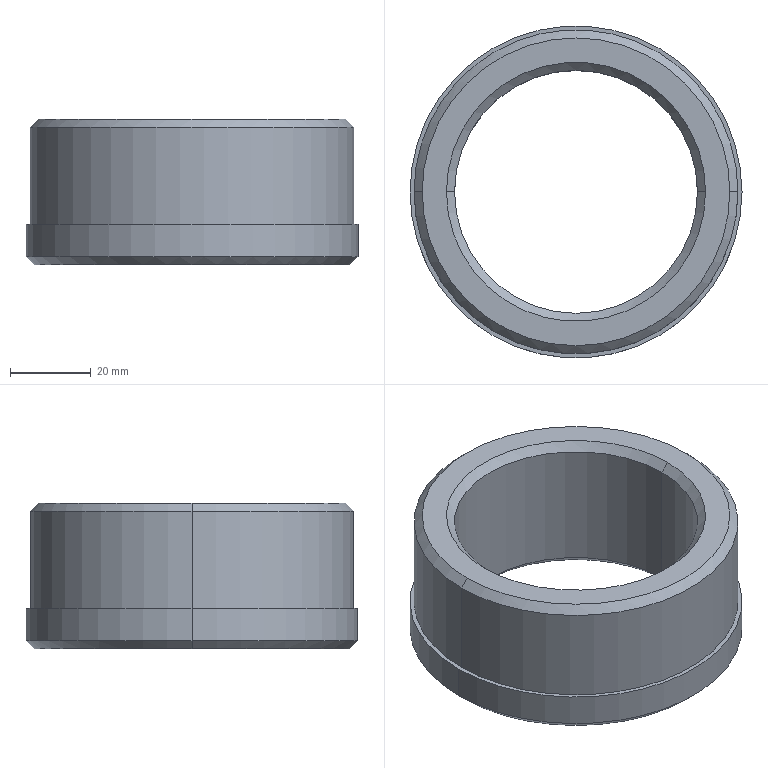Part | SolidWorks | features Chamfer 1, Revolution 1 | 1 solid | 17 faces | box 82 x 82 x 36 mm | volume 79941 mm3 | cone 8 | cylinder 6 | plane 3 | commonest cylinder face diameters 60 x2 80 x2 82 x2
STEP:
#1=CARTESIAN_POINT('',(38.,0.,36.));
#2=VERTEX_POINT('',#1);
#3=CARTESIAN_POINT('',(-38.,0.,36.));
#4=VERTEX_POINT('',#3);
#5=CARTESIAN_POINT('',(0.,0.,36.));
#6=DIRECTION('',(0.,0.,1.));
#7=DIRECTION('',(-1.,0.,0.));
#8=AXIS2_PLACEMENT_3D('',#5,#6,#7);
#9=CIRCLE('',#8,38.);
#10=EDGE_CURVE('',#2,#4,#9,.T.);
#11=ORIENTED_EDGE('',*,*,#10,.F.);
#12=CARTESIAN_POINT('',(40.,0.,34.));
#13=VERTEX_POINT('',#12);
#14=CARTESIAN_POINT('',(40.,0.,34.));
#15=DIRECTION('',(0.7071,0.,-0.7071));
#16=VECTOR('',#15,1000.);
#17=LINE('',#14,#16);
#18=EDGE_CURVE('',#2,#13,#17,.T.);
#19=ORIENTED_EDGE('',*,*,#18,.T.);
#20=CARTESIAN_POINT('',(-40.,0.,34.));
#21=VERTEX_POINT('',#20);
#22=CARTESIAN_POINT('',(0.,0.,34.));
#23=DIRECTION('',(0.,0.,-1.));
#24=DIRECTION('',(-1.,0.,0.));
#25=AXIS2_PLACEMENT_3D('',#22,#23,#24);
#26=CIRCLE('',#25,40.);
#27=EDGE_CURVE('',#21,#13,#26,.T.);
#28=ORIENTED_EDGE('',*,*,#27,.F.);
#29=CARTESIAN_POINT('',(-40.,0.,34.));
#30=DIRECTION('',(-0.7071,0.,-0.7071));
#31=VECTOR('',#30,1000.);
#32=LINE('',#29,#31);
#33=EDGE_CURVE('',#4,#21,#32,.T.);
#34=ORIENTED_EDGE('',*,*,#33,.F.);
#35=EDGE_LOOP('',(#11,#19,#28,#34));
#36=FACE_OUTER_BOUND('',#35,.T.);
#37=CARTESIAN_POINT('',(0.,0.,34.));
#38=DIRECTION('',(0.,0.,-1.));
#39=DIRECTION('',(-1.,0.,0.));
#40=AXIS2_PLACEMENT_3D('',#37,#38,#39);
#41=CONICAL_SURFACE('',#40,40.,0.7854);
#42=ADVANCED_FACE('',(#36),#41,.T.);
#43=CARTESIAN_POINT('',(-30.,0.,34.));
#44=VERTEX_POINT('',#43);
#45=CARTESIAN_POINT('',(30.,0.,34.));
#46=VERTEX_POINT('',#45);
#47=CARTESIAN_POINT('',(0.,0.,34.));
#48=DIRECTION('',(0.,0.,1.));
#49=DIRECTION('',(-1.,0.,0.));
#50=AXIS2_PLACEMENT_3D('',#47,#48,#49);
#51=CIRCLE('',#50,30.);
#52=EDGE_CURVE('',#44,#46,#51,.T.);
#53=ORIENTED_EDGE('',*,*,#52,.F.);
#54=CARTESIAN_POINT('',(-32.,0.,36.));
#55=VERTEX_POINT('',#54);
#56=CARTESIAN_POINT('',(-32.,0.,36.));
#57=DIRECTION('',(-0.7071,0.,0.7071));
#58=VECTOR('',#57,1000.);
#59=LINE('',#56,#58);
#60=EDGE_CURVE('',#44,#55,#59,.T.);
#61=ORIENTED_EDGE('',*,*,#60,.T.);
#62=CARTESIAN_POINT('',(32.,0.,36.));
#63=VERTEX_POINT('',#62);
#64=CARTESIAN_POINT('',(0.,0.,36.));
#65=DIRECTION('',(0.,0.,-1.));
#66=DIRECTION('',(-1.,0.,0.));
#67=AXIS2_PLACEMENT_3D('',#64,#65,#66);
#68=CIRCLE('',#67,32.);
#69=EDGE_CURVE('',#63,#55,#68,.T.);
#70=ORIENTED_EDGE('',*,*,#69,.F.);
#71=CARTESIAN_POINT('',(32.,0.,36.));
#72=DIRECTION('',(0.7071,0.,0.7071));
#73=VECTOR('',#72,1000.);
#74=LINE('',#71,#73);
#75=EDGE_CURVE('',#46,#63,#74,.T.);
#76=ORIENTED_EDGE('',*,*,#75,.F.);
#77=EDGE_LOOP('',(#53,#61,#70,#76));
#78=FACE_OUTER_BOUND('',#77,.T.);
#79=CARTESIAN_POINT('',(0.,0.,36.));
#80=DIRECTION('',(0.,0.,1.));
#81=DIRECTION('',(1.,0.,0.));
#82=AXIS2_PLACEMENT_3D('',#79,#80,#81);
#83=CONICAL_SURFACE('',#82,32.,0.7854);
#84=ADVANCED_FACE('',(#78),#83,.F.);
#85=CARTESIAN_POINT('',(-39.,0.,0.));
#86=VERTEX_POINT('',#85);
#87=CARTESIAN_POINT('',(39.,0.,0.));
#88=VERTEX_POINT('',#87);
#89=CARTESIAN_POINT('',(0.,0.,0.));
#90=DIRECTION('',(0.,0.,-1.));
#91=DIRECTION('',(-1.,0.,0.));
#92=AXIS2_PLACEMENT_3D('',#89,#90,#91);
#93=CIRCLE('',#92,39.);
#94=EDGE_CURVE('',#86,#88,#93,.T.);
#95=ORIENTED_EDGE('',*,*,#94,.F.);
#96=CARTESIAN_POINT('',(-41.,0.,2.));
#97=VERTEX_POINT('',#96);
#98=CARTESIAN_POINT('',(-39.,0.,0.));
#99=DIRECTION('',(-0.7071,0.,0.7071));
#100=VECTOR('',#99,1000.);
#101=LINE('',#98,#100);
#102=EDGE_CURVE('',#86,#97,#101,.T.);
#103=ORIENTED_EDGE('',*,*,#102,.T.);
#104=CARTESIAN_POINT('',(41.,0.,2.));
#105=VERTEX_POINT('',#104);
#106=CARTESIAN_POINT('',(0.,0.,2.));
#107=DIRECTION('',(0.,0.,1.));
#108=DIRECTION('',(-1.,0.,0.));
#109=AXIS2_PLACEMENT_3D('',#106,#107,#108);
#110=CIRCLE('',#109,41.);
#111=EDGE_CURVE('',#105,#97,#110,.T.);
#112=ORIENTED_EDGE('',*,*,#111,.F.);
#113=CARTESIAN_POINT('',(39.,0.,0.));
#114=DIRECTION('',(0.7071,0.,0.7071));
#115=VECTOR('',#114,1000.);
#116=LINE('',#113,#115);
#117=EDGE_CURVE('',#88,#105,#116,.T.);
#118=ORIENTED_EDGE('',*,*,#117,.F.);
#119=EDGE_LOOP('',(#95,#103,#112,#118));
#120=FACE_OUTER_BOUND('',#119,.T.);
#121=CARTESIAN_POINT('',(0.,0.,0.));
#122=DIRECTION('',(0.,0.,1.));
#123=DIRECTION('',(1.,0.,0.));
#124=AXIS2_PLACEMENT_3D('',#121,#122,#123);
#125=CONICAL_SURFACE('',#124,39.,0.7854);
#126=ADVANCED_FACE('',(#120),#125,.T.);
#127=CARTESIAN_POINT('',(30.,0.,2.));
#128=VERTEX_POINT('',#127);
#129=CARTESIAN_POINT('',(-30.,0.,2.));
#130=VERTEX_POINT('',#129);
#131=CARTESIAN_POINT('',(0.,0.,2.));
#132=DIRECTION('',(0.,0.,-1.));
#133=DIRECTION('',(-1.,0.,0.));
#134=AXIS2_PLACEMENT_3D('',#131,#132,#133);
#135=CIRCLE('',#134,30.);
#136=EDGE_CURVE('',#128,#130,#135,.T.);
#137=ORIENTED_EDGE('',*,*,#136,.F.);
#138=CARTESIAN_POINT('',(32.,0.,0.));
#139=VERTEX_POINT('',#138);
#140=CARTESIAN_POINT('',(30.,0.,2.));
#141=DIRECTION('',(0.7071,0.,-0.7071));
#142=VECTOR('',#141,1000.);
#143=LINE('',#140,#142);
#144=EDGE_CURVE('',#128,#139,#143,.T.);
#145=ORIENTED_EDGE('',*,*,#144,.T.);
#146=CARTESIAN_POINT('',(-32.,0.,0.));
#147=VERTEX_POINT('',#146);
#148=CARTESIAN_POINT('',(0.,0.,0.));
#149=DIRECTION('',(0.,0.,1.));
#150=DIRECTION('',(-1.,0.,0.));
#151=AXIS2_PLACEMENT_3D('',#148,#149,#150);
#152=CIRCLE('',#151,32.);
#153=EDGE_CURVE('',#147,#139,#152,.T.);
#154=ORIENTED_EDGE('',*,*,#153,.F.);
#155=CARTESIAN_POINT('',(-30.,0.,2.));
#156=DIRECTION('',(-0.7071,0.,-0.7071));
#157=VECTOR('',#156,1000.);
#158=LINE('',#155,#157);
#159=EDGE_CURVE('',#130,#147,#158,.T.);
#160=ORIENTED_EDGE('',*,*,#159,.F.);
#161=EDGE_LOOP('',(#137,#145,#154,#160));
#162=FACE_OUTER_BOUND('',#161,.T.);
#163=CARTESIAN_POINT('',(0.,0.,2.));
#164=DIRECTION('',(0.,0.,-1.));
#165=DIRECTION('',(-1.,0.,0.));
#166=AXIS2_PLACEMENT_3D('',#163,#164,#165);
#167=CONICAL_SURFACE('',#166,30.,0.7854);
#168=ADVANCED_FACE('',(#162),#167,.F.);
#169=ORIENTED_EDGE('',*,*,#27,.T.);
#170=CARTESIAN_POINT('',(40.,0.,10.));
#171=VERTEX_POINT('',#170);
#172=CARTESIAN_POINT('',(40.,0.,0.));
#173=DIRECTION('',(0.,0.,-1.));
#174=VECTOR('',#173,1000.);
#175=LINE('',#172,#174);
#176=EDGE_CURVE('',#13,#171,#175,.T.);
#177=ORIENTED_EDGE('',*,*,#176,.T.);
#178=CARTESIAN_POINT('',(-40.,0.,10.));
#179=VERTEX_POINT('',#178);
#180=CARTESIAN_POINT('',(0.,0.,10.));
#181=DIRECTION('',(0.,0.,-1.));
#182=DIRECTION('',(-1.,0.,0.));
#183=AXIS2_PLACEMENT_3D('',#180,#181,#182);
#184=CIRCLE('',#183,40.);
#185=EDGE_CURVE('',#179,#171,#184,.T.);
#186=ORIENTED_EDGE('',*,*,#185,.F.);
#187=CARTESIAN_POINT('',(-40.,0.,0.));
#188=DIRECTION('',(0.,0.,-1.));
#189=VECTOR('',#188,1000.);
#190=LINE('',#187,#189);
#191=EDGE_CURVE('',#21,#179,#190,.T.);
#192=ORIENTED_EDGE('',*,*,#191,.F.);
#193=EDGE_LOOP('',(#169,#177,#186,#192));
#194=FACE_OUTER_BOUND('',#193,.T.);
#195=CARTESIAN_POINT('',(0.,0.,0.));
#196=DIRECTION('',(0.,0.,-1.));
#197=DIRECTION('',(-1.,0.,0.));
#198=AXIS2_PLACEMENT_3D('',#195,#196,#197);
#199=CYLINDRICAL_SURFACE('',#198,40.);
#200=ADVANCED_FACE('',(#194),#199,.T.);
#201=CARTESIAN_POINT('',(-41.,0.,10.));
#202=VERTEX_POINT('',#201);
#203=CARTESIAN_POINT('',(41.,0.,10.));
#204=VERTEX_POINT('',#203);
#205=CARTESIAN_POINT('',(0.,0.,10.));
#206=DIRECTION('',(0.,0.,-1.));
#207=DIRECTION('',(-1.,0.,0.));
#208=AXIS2_PLACEMENT_3D('',#205,#206,#207);
#209=CIRCLE('',#208,41.);
#210=EDGE_CURVE('',#202,#204,#209,.T.);
#211=ORIENTED_EDGE('',*,*,#210,.T.);
#212=CARTESIAN_POINT('',(41.,0.,0.));
#213=DIRECTION('',(0.,0.,-1.));
#214=VECTOR('',#213,1000.);
#215=LINE('',#212,#214);
#216=EDGE_CURVE('',#204,#105,#215,.T.);
#217=ORIENTED_EDGE('',*,*,#216,.T.);
#218=ORIENTED_EDGE('',*,*,#111,.T.);
#219=CARTESIAN_POINT('',(-41.,0.,0.));
#220=DIRECTION('',(0.,0.,-1.));
#221=VECTOR('',#220,1000.);
#222=LINE('',#219,#221);
#223=EDGE_CURVE('',#202,#97,#222,.T.);
#224=ORIENTED_EDGE('',*,*,#223,.F.);
#225=EDGE_LOOP('',(#211,#217,#218,#224));
#226=FACE_OUTER_BOUND('',#225,.T.);
#227=CARTESIAN_POINT('',(0.,0.,0.));
#228=DIRECTION('',(0.,0.,-1.));
#229=DIRECTION('',(-1.,0.,0.));
#230=AXIS2_PLACEMENT_3D('',#227,#228,#229);
#231=CYLINDRICAL_SURFACE('',#230,41.);
#232=ADVANCED_FACE('',(#226),#231,.T.);
#233=ORIENTED_EDGE('',*,*,#52,.T.);
#234=CARTESIAN_POINT('',(30.,0.,0.));
#235=DIRECTION('',(0.,0.,-1.));
#236=VECTOR('',#235,1000.);
#237=LINE('',#234,#236);
#238=EDGE_CURVE('',#46,#128,#237,.T.);
#239=ORIENTED_EDGE('',*,*,#238,.T.);
#240=ORIENTED_EDGE('',*,*,#136,.T.);
#241=CARTESIAN_POINT('',(-30.,0.,0.));
#242=DIRECTION('',(0.,0.,-1.));
#243=VECTOR('',#242,1000.);
#244=LINE('',#241,#243);
#245=EDGE_CURVE('',#44,#130,#244,.T.);
#246=ORIENTED_EDGE('',*,*,#245,.F.);
#247=EDGE_LOOP('',(#233,#239,#240,#246));
#248=FACE_OUTER_BOUND('',#247,.T.);
#249=CARTESIAN_POINT('',(0.,0.,0.));
#250=DIRECTION('',(0.,0.,-1.));
#251=DIRECTION('',(-1.,0.,0.));
#252=AXIS2_PLACEMENT_3D('',#249,#250,#251);
#253=CYLINDRICAL_SURFACE('',#252,30.);
#254=ADVANCED_FACE('',(#248),#253,.F.);
#255=ORIENTED_EDGE('',*,*,#238,.F.);
#256=CARTESIAN_POINT('',(0.,0.,34.));
#257=DIRECTION('',(0.,0.,1.));
#258=DIRECTION('',(-1.,0.,0.));
#259=AXIS2_PLACEMENT_3D('',#256,#257,#258);
#260=CIRCLE('',#259,30.);
#261=EDGE_CURVE('',#46,#44,#260,.T.);
#262=ORIENTED_EDGE('',*,*,#261,.T.);
#263=ORIENTED_EDGE('',*,*,#245,.T.);
#264=CARTESIAN_POINT('',(0.,0.,2.));
#265=DIRECTION('',(0.,0.,-1.));
#266=DIRECTION('',(-1.,0.,0.));
#267=AXIS2_PLACEMENT_3D('',#264,#265,#266);
#268=CIRCLE('',#267,30.);
#269=EDGE_CURVE('',#130,#128,#268,.T.);
#270=ORIENTED_EDGE('',*,*,#269,.T.);
#271=EDGE_LOOP('',(#255,#262,#263,#270));
#272=FACE_OUTER_BOUND('',#271,.T.);
#273=CARTESIAN_POINT('',(0.,0.,0.));
#274=DIRECTION('',(0.,0.,-1.));
#275=DIRECTION('',(-1.,0.,0.));
#276=AXIS2_PLACEMENT_3D('',#273,#274,#275);
#277=CYLINDRICAL_SURFACE('',#276,30.);
#278=ADVANCED_FACE('',(#272),#277,.F.);
#279=ORIENTED_EDGE('',*,*,#153,.T.);
#280=CARTESIAN_POINT('',(0.,0.,0.));
#281=DIRECTION('',(0.,0.,1.));
#282=DIRECTION('',(-1.,0.,0.));
#283=AXIS2_PLACEMENT_3D('',#280,#281,#282);
#284=CIRCLE('',#283,32.);
#285=EDGE_CURVE('',#139,#147,#284,.T.);
#286=ORIENTED_EDGE('',*,*,#285,.T.);
#287=EDGE_LOOP('',(#279,#286));
#288=FACE_BOUND('',#287,.T.);
#289=CARTESIAN_POINT('',(0.,0.,0.));
#290=DIRECTION('',(0.,0.,-1.));
#291=DIRECTION('',(-1.,0.,0.));
#292=AXIS2_PLACEMENT_3D('',#289,#290,#291);
#293=CIRCLE('',#292,39.);
#294=EDGE_CURVE('',#88,#86,#293,.T.);
#295=ORIENTED_EDGE('',*,*,#294,.T.);
#296=ORIENTED_EDGE('',*,*,#94,.T.);
#297=EDGE_LOOP('',(#295,#296));
#298=FACE_OUTER_BOUND('',#297,.T.);
#299=CARTESIAN_POINT('',(0.,0.,0.));
#300=DIRECTION('',(0.,0.,-1.));
#301=DIRECTION('',(-1.,0.,0.));
#302=AXIS2_PLACEMENT_3D('',#299,#300,#301);
#303=PLANE('',#302);
#304=ADVANCED_FACE('',(#288,#298),#303,.T.);
#305=ORIENTED_EDGE('',*,*,#216,.F.);
#306=CARTESIAN_POINT('',(0.,0.,10.));
#307=DIRECTION('',(0.,0.,-1.));
#308=DIRECTION('',(-1.,0.,0.));
#309=AXIS2_PLACEMENT_3D('',#306,#307,#308);
#310=CIRCLE('',#309,41.);
#311=EDGE_CURVE('',#204,#202,#310,.T.);
#312=ORIENTED_EDGE('',*,*,#311,.T.);
#313=ORIENTED_EDGE('',*,*,#223,.T.);
#314=CARTESIAN_POINT('',(0.,0.,2.));
#315=DIRECTION('',(0.,0.,1.));
#316=DIRECTION('',(-1.,0.,0.));
#317=AXIS2_PLACEMENT_3D('',#314,#315,#316);
#318=CIRCLE('',#317,41.);
#319=EDGE_CURVE('',#97,#105,#318,.T.);
#320=ORIENTED_EDGE('',*,*,#319,.T.);
#321=EDGE_LOOP('',(#305,#312,#313,#320));
#322=FACE_OUTER_BOUND('',#321,.T.);
#323=CARTESIAN_POINT('',(0.,0.,0.));
#324=DIRECTION('',(0.,0.,-1.));
#325=DIRECTION('',(-1.,0.,0.));
#326=AXIS2_PLACEMENT_3D('',#323,#324,#325);
#327=CYLINDRICAL_SURFACE('',#326,41.);
#328=ADVANCED_FACE('',(#322),#327,.T.);
#329=ORIENTED_EDGE('',*,*,#210,.F.);
#330=ORIENTED_EDGE('',*,*,#311,.F.);
#331=EDGE_LOOP('',(#329,#330));
#332=FACE_OUTER_BOUND('',#331,.T.);
#333=ORIENTED_EDGE('',*,*,#185,.T.);
#334=CARTESIAN_POINT('',(0.,0.,10.));
#335=DIRECTION('',(0.,0.,-1.));
#336=DIRECTION('',(-1.,0.,0.));
#337=AXIS2_PLACEMENT_3D('',#334,#335,#336);
#338=CIRCLE('',#337,40.);
#339=EDGE_CURVE('',#171,#179,#338,.T.);
#340=ORIENTED_EDGE('',*,*,#339,.T.);
#341=EDGE_LOOP('',(#333,#340));
#342=FACE_BOUND('',#341,.T.);
#343=CARTESIAN_POINT('',(0.,0.,10.));
#344=DIRECTION('',(0.,0.,-1.));
#345=DIRECTION('',(-1.,0.,0.));
#346=AXIS2_PLACEMENT_3D('',#343,#344,#345);
#347=PLANE('',#346);
#348=ADVANCED_FACE('',(#332,#342),#347,.F.);
#349=ORIENTED_EDGE('',*,*,#176,.F.);
#350=CARTESIAN_POINT('',(0.,0.,34.));
#351=DIRECTION('',(0.,0.,-1.));
#352=DIRECTION('',(-1.,0.,0.));
#353=AXIS2_PLACEMENT_3D('',#350,#351,#352);
#354=CIRCLE('',#353,40.);
#355=EDGE_CURVE('',#13,#21,#354,.T.);
#356=ORIENTED_EDGE('',*,*,#355,.T.);
#357=ORIENTED_EDGE('',*,*,#191,.T.);
#358=ORIENTED_EDGE('',*,*,#339,.F.);
#359=EDGE_LOOP('',(#349,#356,#357,#358));
#360=FACE_OUTER_BOUND('',#359,.T.);
#361=CARTESIAN_POINT('',(0.,0.,0.));
#362=DIRECTION('',(0.,0.,-1.));
#363=DIRECTION('',(-1.,0.,0.));
#364=AXIS2_PLACEMENT_3D('',#361,#362,#363);
#365=CYLINDRICAL_SURFACE('',#364,40.);
#366=ADVANCED_FACE('',(#360),#365,.T.);
#367=ORIENTED_EDGE('',*,*,#69,.T.);
#368=CARTESIAN_POINT('',(0.,0.,36.));
#369=DIRECTION('',(0.,0.,-1.));
#370=DIRECTION('',(-1.,0.,0.));
#371=AXIS2_PLACEMENT_3D('',#368,#369,#370);
#372=CIRCLE('',#371,32.);
#373=EDGE_CURVE('',#55,#63,#372,.T.);
#374=ORIENTED_EDGE('',*,*,#373,.T.);
#375=EDGE_LOOP('',(#367,#374));
#376=FACE_BOUND('',#375,.T.);
#377=CARTESIAN_POINT('',(0.,0.,36.));
#378=DIRECTION('',(0.,0.,1.));
#379=DIRECTION('',(-1.,0.,0.));
#380=AXIS2_PLACEMENT_3D('',#377,#378,#379);
#381=CIRCLE('',#380,38.);
#382=EDGE_CURVE('',#4,#2,#381,.T.);
#383=ORIENTED_EDGE('',*,*,#382,.T.);
#384=ORIENTED_EDGE('',*,*,#10,.T.);
#385=EDGE_LOOP('',(#383,#384));
#386=FACE_OUTER_BOUND('',#385,.T.);
#387=CARTESIAN_POINT('',(0.,0.,36.));
#388=DIRECTION('',(0.,0.,-1.));
#389=DIRECTION('',(-1.,0.,0.));
#390=AXIS2_PLACEMENT_3D('',#387,#388,#389);
#391=PLANE('',#390);
#392=ADVANCED_FACE('',(#376,#386),#391,.F.);
#393=ORIENTED_EDGE('',*,*,#144,.F.);
#394=ORIENTED_EDGE('',*,*,#269,.F.);
#395=ORIENTED_EDGE('',*,*,#159,.T.);
#396=ORIENTED_EDGE('',*,*,#285,.F.);
#397=EDGE_LOOP('',(#393,#394,#395,#396));
#398=FACE_OUTER_BOUND('',#397,.T.);
#399=CARTESIAN_POINT('',(0.,0.,2.));
#400=DIRECTION('',(0.,0.,-1.));
#401=DIRECTION('',(-1.,0.,0.));
#402=AXIS2_PLACEMENT_3D('',#399,#400,#401);
#403=CONICAL_SURFACE('',#402,30.,0.7854);
#404=ADVANCED_FACE('',(#398),#403,.F.);
#405=ORIENTED_EDGE('',*,*,#102,.F.);
#406=ORIENTED_EDGE('',*,*,#294,.F.);
#407=ORIENTED_EDGE('',*,*,#117,.T.);
#408=ORIENTED_EDGE('',*,*,#319,.F.);
#409=EDGE_LOOP('',(#405,#406,#407,#408));
#410=FACE_OUTER_BOUND('',#409,.T.);
#411=CARTESIAN_POINT('',(0.,0.,0.));
#412=DIRECTION('',(0.,0.,1.));
#413=DIRECTION('',(1.,0.,0.));
#414=AXIS2_PLACEMENT_3D('',#411,#412,#413);
#415=CONICAL_SURFACE('',#414,39.,0.7854);
#416=ADVANCED_FACE('',(#410),#415,.T.);
#417=ORIENTED_EDGE('',*,*,#60,.F.);
#418=ORIENTED_EDGE('',*,*,#261,.F.);
#419=ORIENTED_EDGE('',*,*,#75,.T.);
#420=ORIENTED_EDGE('',*,*,#373,.F.);
#421=EDGE_LOOP('',(#417,#418,#419,#420));
#422=FACE_OUTER_BOUND('',#421,.T.);
#423=CARTESIAN_POINT('',(0.,0.,36.));
#424=DIRECTION('',(0.,0.,1.));
#425=DIRECTION('',(1.,0.,0.));
#426=AXIS2_PLACEMENT_3D('',#423,#424,#425);
#427=CONICAL_SURFACE('',#426,32.,0.7854);
#428=ADVANCED_FACE('',(#422),#427,.F.);
#429=ORIENTED_EDGE('',*,*,#18,.F.);
#430=ORIENTED_EDGE('',*,*,#382,.F.);
#431=ORIENTED_EDGE('',*,*,#33,.T.);
#432=ORIENTED_EDGE('',*,*,#355,.F.);
#433=EDGE_LOOP('',(#429,#430,#431,#432));
#434=FACE_OUTER_BOUND('',#433,.T.);
#435=CARTESIAN_POINT('',(0.,0.,34.));
#436=DIRECTION('',(0.,0.,-1.));
#437=DIRECTION('',(-1.,0.,0.));
#438=AXIS2_PLACEMENT_3D('',#435,#436,#437);
#439=CONICAL_SURFACE('',#438,40.,0.7854);
#440=ADVANCED_FACE('',(#434),#439,.T.);
#441=CLOSED_SHELL('',(#42,#84,#126,#168,#200,#232,#254,#278,#304,#328,#348,#366,#392,#404,#416,#428,#440));
#442=MANIFOLD_SOLID_BREP('',#441);
#443=CARTESIAN_POINT('',(0.,0.,0.));
#444=DIRECTION('',(0.,0.,1.));
#445=DIRECTION('',(1.,0.,0.));
#446=AXIS2_PLACEMENT_3D('',#443,#444,#445);
#447=(LENGTH_UNIT()NAMED_UNIT(*)SI_UNIT(.MILLI.,.METRE.));
#448=UNCERTAINTY_MEASURE_WITH_UNIT(LENGTH_MEASURE(0.00001),#447,'','');
#449=(NAMED_UNIT(*)PLANE_ANGLE_UNIT()SI_UNIT($,.RADIAN.));
#450=(NAMED_UNIT(*)SI_UNIT($,.STERADIAN.)SOLID_ANGLE_UNIT());
#451=(GEOMETRIC_REPRESENTATION_CONTEXT(3)GLOBAL_UNCERTAINTY_ASSIGNED_CONTEXT((#448))GLOBAL_UNIT_ASSIGNED_CONTEXT((#447,#449,#450))REPRESENTATION_CONTEXT('',''));
#452=ADVANCED_BREP_SHAPE_REPRESENTATION('',(#442,#446),#451);